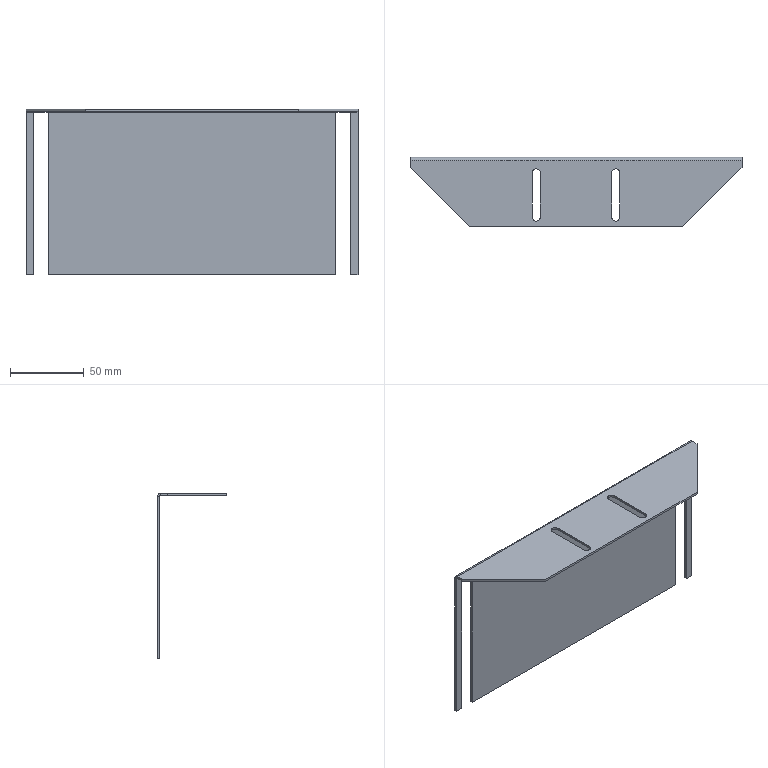Part | STEP file | A14-057 | 1 solid | 36 faces | box 225 x 47 x 112.237 mm | volume 46754 mm3 | plane 30 | cylinder 6 | commonest cylinder face diameters 5.5 x4 1.473 x1 4.473 x1